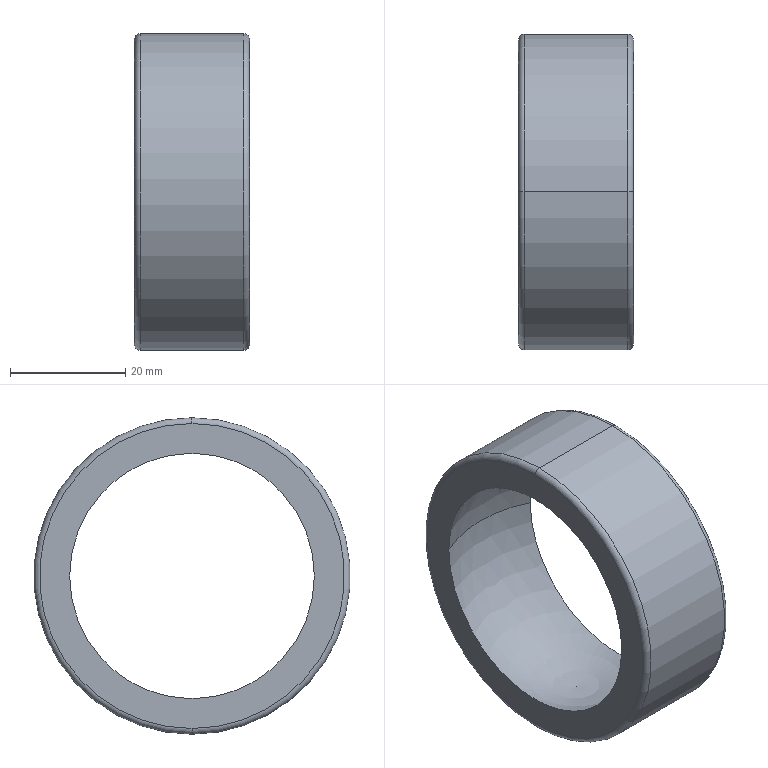Part | SolidWorks | features Fillet 1, Revolution 1 | 1 solid | 10 faces | box 20 x 55 x 55 mm | volume 14839 mm3 | torus 4 | sphere 2 | cylinder 2 | plane 2 | commonest cylinder face diameters 55 x2
STEP:
#1=CARTESIAN_POINT('',(-10.,0.,26.5));
#2=VERTEX_POINT('',#1);
#3=CARTESIAN_POINT('',(-10.,0.,-26.5));
#4=VERTEX_POINT('',#3);
#5=CARTESIAN_POINT('',(-10.,0.,0.));
#6=DIRECTION('',(-1.,0.,0.));
#7=DIRECTION('',(0.,0.,-1.));
#8=AXIS2_PLACEMENT_3D('',#5,#6,#7);
#9=CIRCLE('',#8,26.5);
#10=EDGE_CURVE('',#2,#4,#9,.T.);
#11=ORIENTED_EDGE('',*,*,#10,.F.);
#12=CARTESIAN_POINT('',(-9.,0.,27.5));
#13=VERTEX_POINT('',#12);
#14=CARTESIAN_POINT('',(-9.,0.,26.5));
#15=DIRECTION('',(0.,1.,0.));
#16=DIRECTION('',(0.,0.,1.));
#17=AXIS2_PLACEMENT_3D('',#14,#15,#16);
#18=CIRCLE('',#17,1.);
#19=EDGE_CURVE('',#2,#13,#18,.T.);
#20=ORIENTED_EDGE('',*,*,#19,.T.);
#21=CARTESIAN_POINT('',(-9.,0.,-27.5));
#22=VERTEX_POINT('',#21);
#23=CARTESIAN_POINT('',(-9.,0.,0.));
#24=DIRECTION('',(1.,0.,0.));
#25=DIRECTION('',(0.,0.,-1.));
#26=AXIS2_PLACEMENT_3D('',#23,#24,#25);
#27=CIRCLE('',#26,27.5);
#28=EDGE_CURVE('',#22,#13,#27,.T.);
#29=ORIENTED_EDGE('',*,*,#28,.F.);
#30=CARTESIAN_POINT('',(-9.,0.,-26.5));
#31=DIRECTION('',(0.,-1.,0.));
#32=DIRECTION('',(0.,0.,-1.));
#33=AXIS2_PLACEMENT_3D('',#30,#31,#32);
#34=CIRCLE('',#33,1.);
#35=EDGE_CURVE('',#4,#22,#34,.T.);
#36=ORIENTED_EDGE('',*,*,#35,.F.);
#37=EDGE_LOOP('',(#11,#20,#29,#36));
#38=FACE_OUTER_BOUND('',#37,.T.);
#39=CARTESIAN_POINT('',(-9.,0.,0.));
#40=DIRECTION('',(1.,0.,0.));
#41=DIRECTION('',(0.,0.,-1.));
#42=AXIS2_PLACEMENT_3D('',#39,#40,#41);
#43=TOROIDAL_SURFACE('',#42,26.5,1.);
#44=ADVANCED_FACE('',(#38),#43,.T.);
#45=CARTESIAN_POINT('',(10.,0.,-26.5));
#46=VERTEX_POINT('',#45);
#47=CARTESIAN_POINT('',(10.,0.,26.5));
#48=VERTEX_POINT('',#47);
#49=CARTESIAN_POINT('',(10.,0.,0.));
#50=DIRECTION('',(1.,0.,0.));
#51=DIRECTION('',(0.,0.,1.));
#52=AXIS2_PLACEMENT_3D('',#49,#50,#51);
#53=CIRCLE('',#52,26.5);
#54=EDGE_CURVE('',#46,#48,#53,.T.);
#55=ORIENTED_EDGE('',*,*,#54,.F.);
#56=CARTESIAN_POINT('',(9.,0.,-27.5));
#57=VERTEX_POINT('',#56);
#58=CARTESIAN_POINT('',(9.,0.,-26.5));
#59=DIRECTION('',(0.,1.,0.));
#60=DIRECTION('',(0.,0.,1.));
#61=AXIS2_PLACEMENT_3D('',#58,#59,#60);
#62=CIRCLE('',#61,1.);
#63=EDGE_CURVE('',#46,#57,#62,.T.);
#64=ORIENTED_EDGE('',*,*,#63,.T.);
#65=CARTESIAN_POINT('',(9.,0.,27.5));
#66=VERTEX_POINT('',#65);
#67=CARTESIAN_POINT('',(9.,0.,0.));
#68=DIRECTION('',(-1.,0.,0.));
#69=DIRECTION('',(0.,0.,1.));
#70=AXIS2_PLACEMENT_3D('',#67,#68,#69);
#71=CIRCLE('',#70,27.5);
#72=EDGE_CURVE('',#66,#57,#71,.T.);
#73=ORIENTED_EDGE('',*,*,#72,.F.);
#74=CARTESIAN_POINT('',(9.,0.,26.5));
#75=DIRECTION('',(0.,-1.,0.));
#76=DIRECTION('',(0.,0.,-1.));
#77=AXIS2_PLACEMENT_3D('',#74,#75,#76);
#78=CIRCLE('',#77,1.);
#79=EDGE_CURVE('',#48,#66,#78,.T.);
#80=ORIENTED_EDGE('',*,*,#79,.F.);
#81=EDGE_LOOP('',(#55,#64,#73,#80));
#82=FACE_OUTER_BOUND('',#81,.T.);
#83=CARTESIAN_POINT('',(9.,0.,0.));
#84=DIRECTION('',(-1.,0.,0.));
#85=DIRECTION('',(0.,0.,1.));
#86=AXIS2_PLACEMENT_3D('',#83,#84,#85);
#87=TOROIDAL_SURFACE('',#86,26.5,1.);
#88=ADVANCED_FACE('',(#82),#87,.T.);
#89=CARTESIAN_POINT('',(10.,-21.266,0.));
#90=VERTEX_POINT('',#89);
#91=CARTESIAN_POINT('',(10.,21.266,0.));
#92=VERTEX_POINT('',#91);
#93=CARTESIAN_POINT('',(10.,0.,0.));
#94=DIRECTION('',(-1.,0.,0.));
#95=DIRECTION('',(0.,0.,1.));
#96=AXIS2_PLACEMENT_3D('',#93,#94,#95);
#97=CIRCLE('',#96,21.266);
#98=EDGE_CURVE('',#90,#92,#97,.T.);
#99=ORIENTED_EDGE('',*,*,#98,.F.);
#100=CARTESIAN_POINT('',(-10.,-21.266,0.));
#101=VERTEX_POINT('',#100);
#102=CARTESIAN_POINT('',(0.,0.,0.));
#103=DIRECTION('',(0.,0.,-1.));
#104=DIRECTION('',(0.,1.,0.));
#105=AXIS2_PLACEMENT_3D('',#102,#103,#104);
#106=CIRCLE('',#105,23.5);
#107=EDGE_CURVE('',#90,#101,#106,.T.);
#108=ORIENTED_EDGE('',*,*,#107,.T.);
#109=CARTESIAN_POINT('',(-10.,21.266,0.));
#110=VERTEX_POINT('',#109);
#111=CARTESIAN_POINT('',(-10.,0.,0.));
#112=DIRECTION('',(-1.,0.,0.));
#113=DIRECTION('',(0.,0.,1.));
#114=AXIS2_PLACEMENT_3D('',#111,#112,#113);
#115=CIRCLE('',#114,21.266);
#116=EDGE_CURVE('',#101,#110,#115,.T.);
#117=ORIENTED_EDGE('',*,*,#116,.T.);
#118=CARTESIAN_POINT('',(0.,0.,0.));
#119=DIRECTION('',(0.,0.,1.));
#120=DIRECTION('',(1.,0.,0.));
#121=AXIS2_PLACEMENT_3D('',#118,#119,#120);
#122=CIRCLE('',#121,23.5);
#123=EDGE_CURVE('',#92,#110,#122,.T.);
#124=ORIENTED_EDGE('',*,*,#123,.F.);
#125=EDGE_LOOP('',(#99,#108,#117,#124));
#126=FACE_OUTER_BOUND('',#125,.T.);
#127=CARTESIAN_POINT('',(0.,0.,0.));
#128=DIRECTION('',(0.,0.,-1.));
#129=DIRECTION('',(0.,1.,0.));
#130=AXIS2_PLACEMENT_3D('',#127,#128,#129);
#131=SPHERICAL_SURFACE('',#130,23.5);
#132=ADVANCED_FACE('',(#126),#131,.F.);
#133=ORIENTED_EDGE('',*,*,#72,.T.);
#134=CARTESIAN_POINT('',(-48.231,0.,-27.5));
#135=DIRECTION('',(-1.,0.,0.));
#136=VECTOR('',#135,1000.);
#137=LINE('',#134,#136);
#138=EDGE_CURVE('',#57,#22,#137,.T.);
#139=ORIENTED_EDGE('',*,*,#138,.T.);
#140=ORIENTED_EDGE('',*,*,#28,.T.);
#141=CARTESIAN_POINT('',(-48.231,0.,27.5));
#142=DIRECTION('',(-1.,0.,0.));
#143=VECTOR('',#142,1000.);
#144=LINE('',#141,#143);
#145=EDGE_CURVE('',#66,#13,#144,.T.);
#146=ORIENTED_EDGE('',*,*,#145,.F.);
#147=EDGE_LOOP('',(#133,#139,#140,#146));
#148=FACE_OUTER_BOUND('',#147,.T.);
#149=CARTESIAN_POINT('',(-48.231,0.,0.));
#150=DIRECTION('',(-1.,0.,0.));
#151=DIRECTION('',(0.,0.,1.));
#152=AXIS2_PLACEMENT_3D('',#149,#150,#151);
#153=CYLINDRICAL_SURFACE('',#152,27.5);
#154=ADVANCED_FACE('',(#148),#153,.T.);
#155=ORIENTED_EDGE('',*,*,#138,.F.);
#156=CARTESIAN_POINT('',(9.,0.,0.));
#157=DIRECTION('',(-1.,0.,0.));
#158=DIRECTION('',(0.,0.,1.));
#159=AXIS2_PLACEMENT_3D('',#156,#157,#158);
#160=CIRCLE('',#159,27.5);
#161=EDGE_CURVE('',#57,#66,#160,.T.);
#162=ORIENTED_EDGE('',*,*,#161,.T.);
#163=ORIENTED_EDGE('',*,*,#145,.T.);
#164=CARTESIAN_POINT('',(-9.,0.,0.));
#165=DIRECTION('',(1.,0.,0.));
#166=DIRECTION('',(0.,0.,-1.));
#167=AXIS2_PLACEMENT_3D('',#164,#165,#166);
#168=CIRCLE('',#167,27.5);
#169=EDGE_CURVE('',#13,#22,#168,.T.);
#170=ORIENTED_EDGE('',*,*,#169,.T.);
#171=EDGE_LOOP('',(#155,#162,#163,#170));
#172=FACE_OUTER_BOUND('',#171,.T.);
#173=CARTESIAN_POINT('',(-48.231,0.,0.));
#174=DIRECTION('',(-1.,0.,0.));
#175=DIRECTION('',(0.,0.,1.));
#176=AXIS2_PLACEMENT_3D('',#173,#174,#175);
#177=CYLINDRICAL_SURFACE('',#176,27.5);
#178=ADVANCED_FACE('',(#172),#177,.T.);
#179=CARTESIAN_POINT('',(-10.,0.,0.));
#180=DIRECTION('',(-1.,0.,0.));
#181=DIRECTION('',(0.,0.,-1.));
#182=AXIS2_PLACEMENT_3D('',#179,#180,#181);
#183=CIRCLE('',#182,26.5);
#184=EDGE_CURVE('',#4,#2,#183,.T.);
#185=ORIENTED_EDGE('',*,*,#184,.T.);
#186=ORIENTED_EDGE('',*,*,#10,.T.);
#187=EDGE_LOOP('',(#185,#186));
#188=FACE_OUTER_BOUND('',#187,.T.);
#189=CARTESIAN_POINT('',(-10.,0.,0.));
#190=DIRECTION('',(-1.,0.,0.));
#191=DIRECTION('',(0.,0.,1.));
#192=AXIS2_PLACEMENT_3D('',#189,#190,#191);
#193=CIRCLE('',#192,21.266);
#194=EDGE_CURVE('',#110,#101,#193,.T.);
#195=ORIENTED_EDGE('',*,*,#194,.F.);
#196=ORIENTED_EDGE('',*,*,#116,.F.);
#197=EDGE_LOOP('',(#195,#196));
#198=FACE_BOUND('',#197,.T.);
#199=CARTESIAN_POINT('',(-10.,27.5,0.));
#200=DIRECTION('',(1.,0.,0.));
#201=DIRECTION('',(0.,0.,-1.));
#202=AXIS2_PLACEMENT_3D('',#199,#200,#201);
#203=PLANE('',#202);
#204=ADVANCED_FACE('',(#188,#198),#203,.F.);
#205=ORIENTED_EDGE('',*,*,#107,.F.);
#206=CARTESIAN_POINT('',(10.,0.,0.));
#207=DIRECTION('',(-1.,0.,0.));
#208=DIRECTION('',(0.,0.,1.));
#209=AXIS2_PLACEMENT_3D('',#206,#207,#208);
#210=CIRCLE('',#209,21.266);
#211=EDGE_CURVE('',#92,#90,#210,.T.);
#212=ORIENTED_EDGE('',*,*,#211,.F.);
#213=ORIENTED_EDGE('',*,*,#123,.T.);
#214=ORIENTED_EDGE('',*,*,#194,.T.);
#215=EDGE_LOOP('',(#205,#212,#213,#214));
#216=FACE_OUTER_BOUND('',#215,.T.);
#217=CARTESIAN_POINT('',(0.,0.,0.));
#218=DIRECTION('',(0.,0.,-1.));
#219=DIRECTION('',(0.,1.,0.));
#220=AXIS2_PLACEMENT_3D('',#217,#218,#219);
#221=SPHERICAL_SURFACE('',#220,23.5);
#222=ADVANCED_FACE('',(#216),#221,.F.);
#223=CARTESIAN_POINT('',(10.,0.,0.));
#224=DIRECTION('',(1.,0.,0.));
#225=DIRECTION('',(0.,0.,1.));
#226=AXIS2_PLACEMENT_3D('',#223,#224,#225);
#227=CIRCLE('',#226,26.5);
#228=EDGE_CURVE('',#48,#46,#227,.T.);
#229=ORIENTED_EDGE('',*,*,#228,.T.);
#230=ORIENTED_EDGE('',*,*,#54,.T.);
#231=EDGE_LOOP('',(#229,#230));
#232=FACE_OUTER_BOUND('',#231,.T.);
#233=ORIENTED_EDGE('',*,*,#211,.T.);
#234=ORIENTED_EDGE('',*,*,#98,.T.);
#235=EDGE_LOOP('',(#233,#234));
#236=FACE_BOUND('',#235,.T.);
#237=CARTESIAN_POINT('',(10.,27.5,0.));
#238=DIRECTION('',(-1.,0.,0.));
#239=DIRECTION('',(0.,0.,1.));
#240=AXIS2_PLACEMENT_3D('',#237,#238,#239);
#241=PLANE('',#240);
#242=ADVANCED_FACE('',(#232,#236),#241,.F.);
#243=ORIENTED_EDGE('',*,*,#63,.F.);
#244=ORIENTED_EDGE('',*,*,#228,.F.);
#245=ORIENTED_EDGE('',*,*,#79,.T.);
#246=ORIENTED_EDGE('',*,*,#161,.F.);
#247=EDGE_LOOP('',(#243,#244,#245,#246));
#248=FACE_OUTER_BOUND('',#247,.T.);
#249=CARTESIAN_POINT('',(9.,0.,0.));
#250=DIRECTION('',(-1.,0.,0.));
#251=DIRECTION('',(0.,0.,1.));
#252=AXIS2_PLACEMENT_3D('',#249,#250,#251);
#253=TOROIDAL_SURFACE('',#252,26.5,1.);
#254=ADVANCED_FACE('',(#248),#253,.T.);
#255=ORIENTED_EDGE('',*,*,#19,.F.);
#256=ORIENTED_EDGE('',*,*,#184,.F.);
#257=ORIENTED_EDGE('',*,*,#35,.T.);
#258=ORIENTED_EDGE('',*,*,#169,.F.);
#259=EDGE_LOOP('',(#255,#256,#257,#258));
#260=FACE_OUTER_BOUND('',#259,.T.);
#261=CARTESIAN_POINT('',(-9.,0.,0.));
#262=DIRECTION('',(1.,0.,0.));
#263=DIRECTION('',(0.,0.,-1.));
#264=AXIS2_PLACEMENT_3D('',#261,#262,#263);
#265=TOROIDAL_SURFACE('',#264,26.5,1.);
#266=ADVANCED_FACE('',(#260),#265,.T.);
#267=CLOSED_SHELL('',(#44,#88,#132,#154,#178,#204,#222,#242,#254,#266));
#268=MANIFOLD_SOLID_BREP('',#267);
#269=CARTESIAN_POINT('',(0.,0.,0.));
#270=DIRECTION('',(0.,0.,1.));
#271=DIRECTION('',(1.,0.,0.));
#272=AXIS2_PLACEMENT_3D('',#269,#270,#271);
#273=(LENGTH_UNIT()NAMED_UNIT(*)SI_UNIT(.MILLI.,.METRE.));
#274=UNCERTAINTY_MEASURE_WITH_UNIT(LENGTH_MEASURE(0.00001),#273,'','');
#275=(NAMED_UNIT(*)PLANE_ANGLE_UNIT()SI_UNIT($,.RADIAN.));
#276=(NAMED_UNIT(*)SI_UNIT($,.STERADIAN.)SOLID_ANGLE_UNIT());
#277=(GEOMETRIC_REPRESENTATION_CONTEXT(3)GLOBAL_UNCERTAINTY_ASSIGNED_CONTEXT((#274))GLOBAL_UNIT_ASSIGNED_CONTEXT((#273,#275,#276))REPRESENTATION_CONTEXT('',''));
#278=ADVANCED_BREP_SHAPE_REPRESENTATION('',(#268,#272),#277);